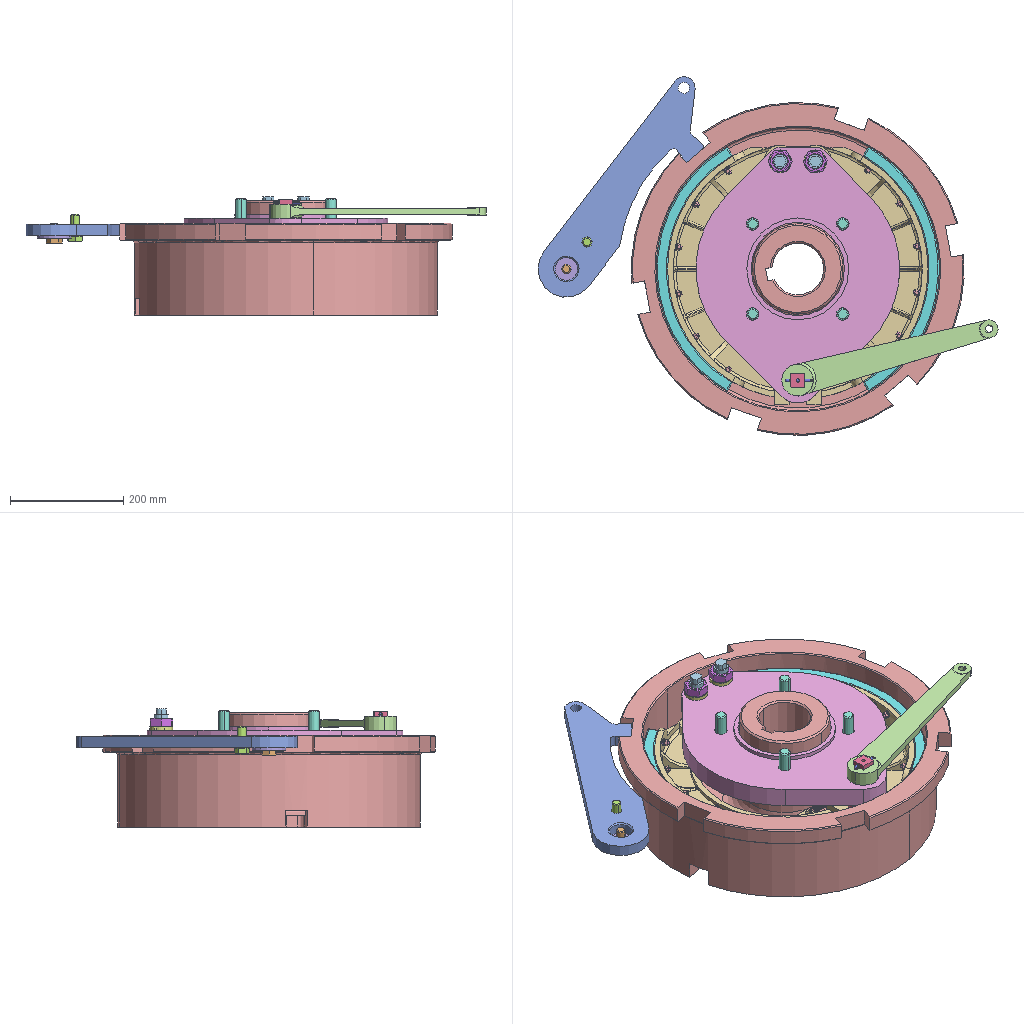Assembly | SolidWorks | 24 different items | 129 placed | box 812 x 633 x 209 mm
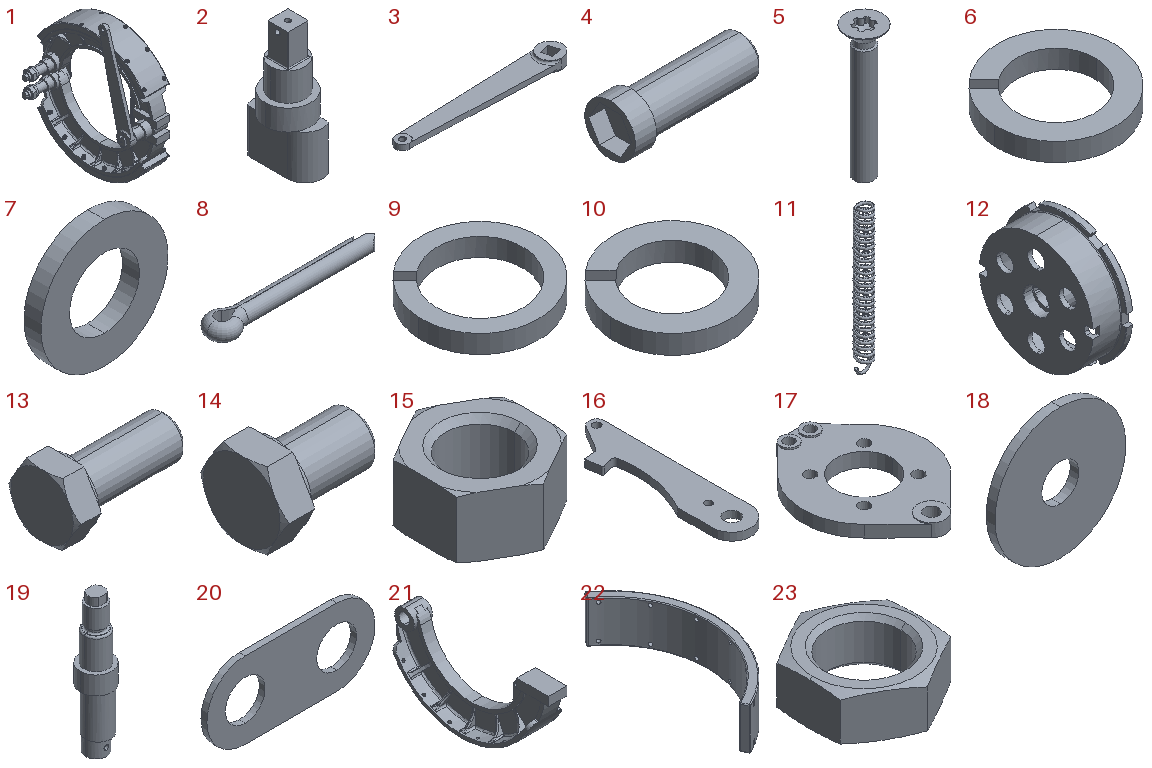Parts list (item | name | quantity | parent item | size | volume | features):
1 | (subassembly) | x1 | - | - | 5849536 mm3 | features ReferencePattern 44, MateUpdatePoint 4, LocalCirPattern 1, LocalLPattern 1, RefAxis 1
2 | - | x1 | in 1 | 55 x 72 x 150 mm | 234412 mm3 | features Boss 3, Chamfer 2, Cut 2, Extrusion 1, Fillet 1
3 | - | x1 | in 1 | 394 x 56 x 25 mm | 222247 mm3 | features Boss 2, Fillet 2, Chamfer 1, Cut 1, Extrusion 1
4 | - | x4 | - | 62.8 x 24 x 24 mm | 17476 mm3 | features Chamfer 1, Cut 1, Extrusion 1, Fillet 1, LPattern 1, RevCut 1, Revolution 1
5 | - | x24 | in 1 | 11.3 x 11.3 x 40 mm | 1175 mm3 | features RevCut 2, Cut 1, Extrusion 1, LPattern 1, Revolution 1
6 | - | x2 | in 1 | 40.929 x 40.929 x 9.844 mm | 4521 mm3 | features Boss 1, Cut 1, Extrusion 1, Helix 1, Sweep 1
7 | - | x24 | in 1 | 12 x 1.6 x 12 mm | 126.217 mm3 | features Revolution 1
8 | - | x3 | in 1 | 50 x 9.2 x 5 mm | 942.558 mm3 | features Cut 1, Sweep 1
9 | - | x4 | - | 30.24 x 30.24 x 7.233 mm | 1507 mm3 | features Boss 1, Cut 1, Extrusion 1, Helix 1, Sweep 1
10 | - | x24 | in 1 | 9.282 x 9.282 x 2.331 mm | 56.214 mm3 | features Boss 1, Cut 1, Extrusion 1, Helix 1, Sweep 1
11 | - | x1 | in 1 | 12 x 12 x 111.085 mm | 2504 mm3 | features Sweep 3, Helix 1, MirrorPattern 1, RefAxis 1
12 | - | x1 | - | 202 x 585.327 x 588 mm | 11095481 mm3 | features Cut 5, Chamfer 3, Fillet 3, Boss 2, CirPattern 2, Extrusion 1, RefAxis 1, RevCut 1
13 | - | x1 | - | 48 x 27.713 x 24 mm | 12520 mm3 | features RevCut 4, Chamfer 1, Extrusion 1, Fillet 1, LPattern 1, Revolution 1
14 | - | x1 | - | 35.4 x 27.713 x 24 mm | 9987 mm3 | features RevCut 4, Chamfer 1, Extrusion 1, Fillet 1, LPattern 1, Revolution 1
15 | - | x24 | in 1 | 9.591 x 11.05 x 5.2 mm | 259.734 mm3 | features Cut 2, Chamfer 1, Extrusion 1
16 | - | x1 | - | 111.471 x 450 x 20 mm | 668870 mm3 | features Fillet 2, Chamfer 1, Extrusion 1
17 | - | x1 | in 1 | 360 x 452 x 47 mm | 3099726 mm3 | features Boss 3, Cut 2, CirPattern 1, Extrusion 1, RefAxis 1
18 | - | x1 | - | 60 x 4 x 60 mm | 10402 mm3 | features Extrusion 1
19 | - | x2 | in 1 | 40 x 40 x 175 mm | 126777 mm3 | features Boss 6, Chamfer 2, Cut 2, Extrusion 1, Fillet 1
20 | - | x1 | in 1 | 114 x 4 x 52 mm | 16810 mm3 | features Extrusion 1
21 | - | x2 | in 1 | 100 x 459 x 228 mm | 1537411 mm3 | features Cut 5, Boss 4, Fillet 4, CirPattern 3, MirrorPattern 2, RefAxis 1, RevCut 1, Revolution 1, Rib 1
22 | - | x2 | in 1 | 152.144 x 429.908 x 100 mm | 988120 mm3 | features CirPattern 1, Cut 1, Extrusion 1, Fillet 1, MirrorPattern 1, RefAxis 1, RevCut 1
23 | - | x2 | in 1 | 37.323 x 43 x 15 mm | 10304 mm3 | features Cut 2, Chamfer 1, Extrusion 1
24 | GR456-00 | x1 | - | - | - | -
Mates (type | each side: item.copy, entity, surface, feature):
In the top assembly
Concentric | 14.1 face cylinder Boss-Revolve1 | 18.1 face cylinder Extrude1
Coincident | 14.1 face plane Base-Extrude | 18.1 face plane Extrude1
Parallel | 14.1 face plane Base-Extrude | 18.1 plane
Concentric | 4.1 face cylinder Boss-Revolve1 | 9.1 face cylinder Boss-Extrude1
Concentric | 16.1 face cylinder Extrude1 | 14.1 face cylinder Boss-Revolve1
Coincident | 16.1 face plane Extrude1 | 18.1 face plane Extrude1
Coincident | 4.1 face plane Base-Extrude | 9.1 face plane Boss-Extrude1
Concentric | 17.1 face cylinder Cut-Extrude9 | 4.1 face cylinder Boss-Revolve1
Coincident | 17.1 face plane Cut-Extrude9 | 9.1 edge
Concentric | 17.1 face cylinder Extrude1 | 19.1 face cylinder Extrude4
Coincident | 19.1 face plane Extrude3 | 17.1 face plane Extrude2
Concentric | 17.1 face cylinder Extrude1 | 19.2 face cylinder Extrude3
Concentric | 16.1 face cylinder Extrude1 | 13.1 face cylinder Boss-Revolve1
Coincident | 16.1 face plane Extrude1 | 13.1 face plane Base-Extrude
Coincident | 1.1 select_type:25 | assembly select_type:11
Coincident | 1.1 plane | assembly plane | 2 times
Concentric | 12.1 face cylinder Cut-Revolve1 | 17.1 face cylinder Extrude1
DistanceDim | 12.1 face plane Cut-Revolve1 | 21.1 face plane Extrude8
DistanceDim | 16.1 select_type:25 | assembly select_type:11
Coincident | 16.1 select_type:25 | assembly plane
DistanceDim | 12.1 face plane Extrude1 | 16.1 face plane Extrude1
Tangent | 12.1 face plane Extrude2 | 16.1 face cylinder Fillet1 | 2 times
In subassembly 1
Concentric | 17.1 face | 2.1 face cylinder Extrude6
Coincident | 17.1 face | 6.1 face plane Boss-Extrude1
Coincident | 23.1 face plane Base-Extrude | 6.1 face plane Base-Extrude
Concentric | 19.3 face cylinder Extrude6 | 6.2 face cylinder Boss-Extrude1
Coincident | 17.1 face | 6.2 face plane Boss-Extrude1
Concentric | 23.2 face cylinder Base-Extrude | 19.3 face cylinder Extrude6
Coincident | 23.2 face plane Base-Extrude | 6.2 face plane Base-Extrude
Concentric | 20.1 face cylinder Extrude1 | 19.3 face cylinder Extrude1
Concentric | 20.1 face cylinder Extrude1 | 19.4 face cylinder Extrude1
Concentric | 8.1 face cylinder Body | 19.3 face cylinder Cut-Extrude1
Tangent | 8.1 plane | 19.3 face cylinder Extrude1
Coincident | 2.1 face plane Extrude5 | 17.1 face
Concentric | 17.1 face | 19.4 face cylinder Extrude4
Concentric | 17.1 face | 19.3 face cylinder Extrude4
Parallel | 17.1 face | 19.4 face plane Extrude7
Coincident | 19.4 face plane Extrude2 | 20.1 face plane Extrude1
Coincident | 19.4 face plane Extrude3 | 17.1 face
Concentric | 19.4 face cylinder Extrude6 | 23.1 face cylinder Base-Extrude
Concentric | 19.4 face cylinder Cut-Extrude1 | 8.2 face cylinder Body
Tangent | 19.4 face cylinder Extrude1 | 8.2 plane
Coincident | 2.1 face plane Extrude4 | 3.1 face plane Cut-Extrude1 | 2 times
Coincident | 17.1 face | 3.1 face plane Extrude2
Concentric | 21.2 face cylinder Mirror11 | 5.1 face cylinder Base-Extrude | 2 times
Concentric | 21.2 face cylinder Revolve1 | 22.1 face cylinder Extrude1
Concentric | 21.2 face cylinder Mirror11 | 22.1 face cylinder Mirror1
Concentric | 21.2 face cylinder Cut-Extrude3 | 19.4 face cylinder Extrude2
Concentric | 21.3 face cylinder Revolve1 | 22.2 face cylinder Extrude1
Concentric | 21.3 face cylinder Mirror11 | 22.2 face cylinder Mirror1
Concentric | 21.3 face cylinder Cut-Extrude3 | 19.3 face cylinder Extrude2
DistanceDim | 11.1 plane | 21.3 face plane Extrude4
Coincident | 19.3 face plane Extrude3 | 21.3 face plane Extrude3
Coincident | 17.1 select_type:0 | 1.2 select_type:11
Coincident | 17.1 plane | 1.2 plane | 3 times
Concentric | 2.1 face cylinder Cut-Extrude2 | 8.3 face cylinder Body
Coincident | 2.1 face plane Extrude4 | 8.3 plane
Parallel | 17.1 face | 2.1 face plane Extrude4
Parallel | 17.1 face | 8.3 plane
Coincident | 19.4 face plane Extrude3 | 21.2 face plane Extrude3
Coincident | 17.1 face | 19.3 face plane Extrude3
DistanceDim | 11.1 plane | 21.3 face plane Extrude6
Tangent | 11.1 face surface:4010 Sweep9 | 21.3 face cylinder Extrude6
Concentric | 19.4 face cylinder Extrude6 | 6.1 face cylinder Boss-Extrude1
Tangent | 21.2 face cylinder Revolve1 | 7.1 face plane Base-Revolve
Coincident | 7.1 face plane Base-Revolve | 10.1 face plane Base-Extrude
Coincident | 10.1 face plane Boss-Extrude1 | 15.1 face plane Base-Extrude
DistanceDim | 5.1 face plane Base-Extrude | 15.1 face plane Base-Extrude
Concentric | 5.1 face cylinder Base-Extrude | 7.1 face cylinder Base-Revolve
Tangent | 2.1 face cylinder Extrude1 | 21.3 face plane Extrude4
Tangent | 2.1 face cylinder Extrude1 | 21.2 face plane Extrude4